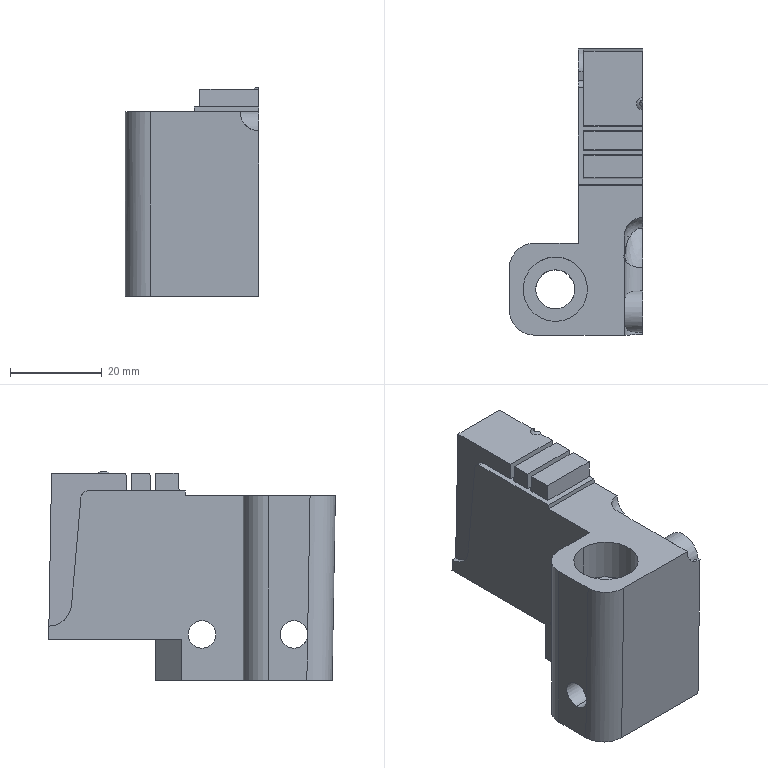Part | Creo | 1 solid | 177 faces | box 29 x 62.341 x 45.424 mm | volume 39599 mm3 | other 95 | plane 57 | cylinder 19 | sphere 3 | spline 2 | cone 1 | commonest cylinder face diameters 6 x6 8 x3 8.5 x2 11 x2 14 x2 3.012 x1